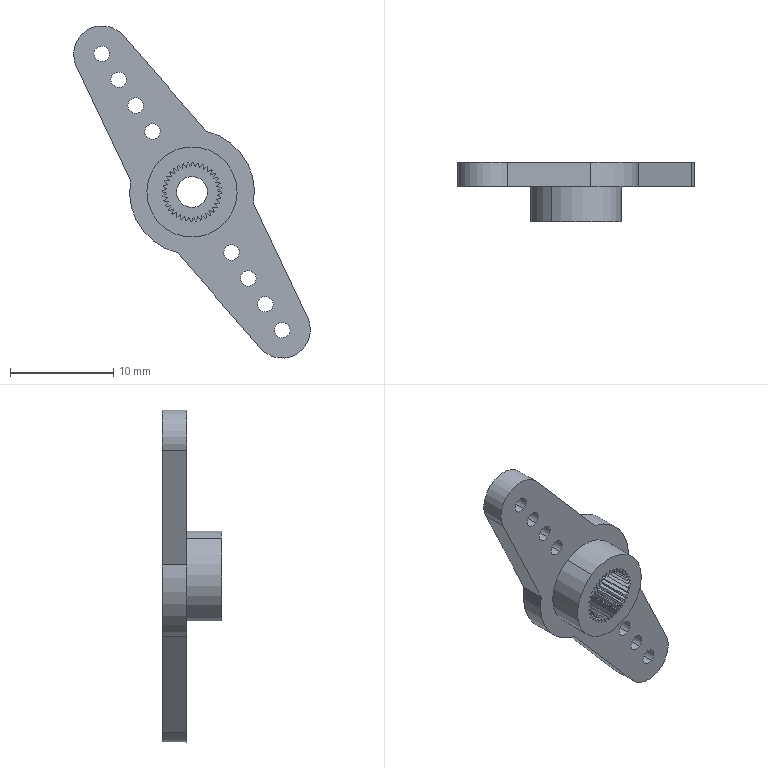Part | SolidWorks | features BaseBody 1 | 1 solid | 150 faces | box 22.948 x 5.75 x 32.206 mm | volume 734.003 mm3 | plane 83 | cylinder 67 | commonest cylinder face diameters 5.7 x36 1.5 x16 5.5 x5 3 x2 6.5 x2 8.75 x2